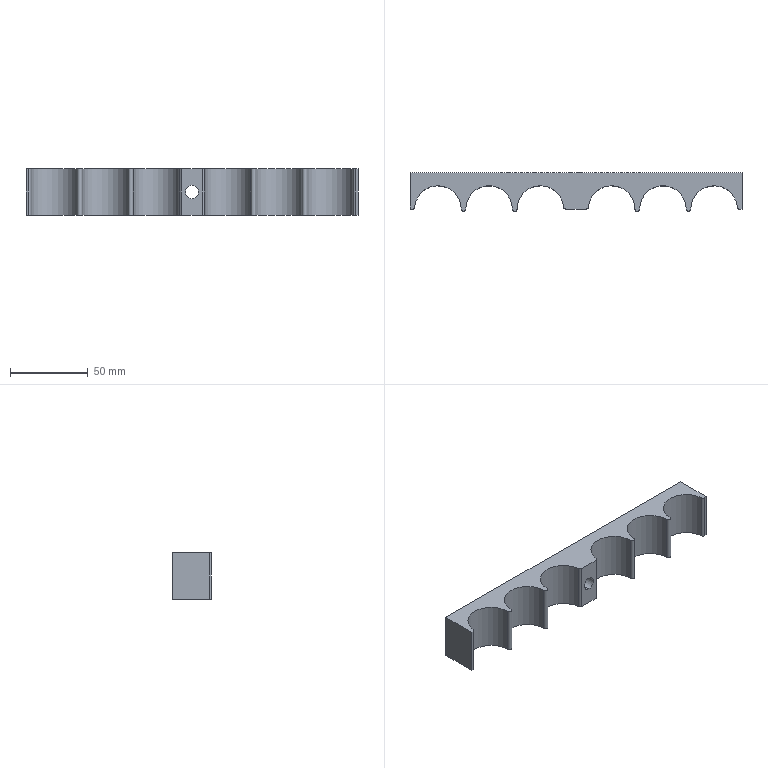Part | SolidWorks | features Extrusion 1, HoleWzd 1 | 1 solid | 24 faces | box 214 x 25 x 30 mm | volume 86293 mm3 | cylinder 16 | plane 8 | commonest cylinder face diameters 3 x8 30 x6 8.5 x2
STEP:
#1=CARTESIAN_POINT('',(0.,0.,10.75));
#2=VERTEX_POINT('',#1);
#3=CARTESIAN_POINT('',(0.,0.,19.25));
#4=VERTEX_POINT('',#3);
#5=CARTESIAN_POINT('',(0.,0.,15.));
#6=DIRECTION('',(0.,1.,0.));
#7=DIRECTION('',(0.,0.,1.));
#8=AXIS2_PLACEMENT_3D('',#5,#6,#7);
#9=CIRCLE('',#8,4.25);
#10=EDGE_CURVE('',#2,#4,#9,.T.);
#11=ORIENTED_EDGE('',*,*,#10,.F.);
#12=CARTESIAN_POINT('',(0.,23.5,10.75));
#13=VERTEX_POINT('',#12);
#14=CARTESIAN_POINT('',(0.,23.5,10.75));
#15=DIRECTION('',(0.,1.,0.));
#16=VECTOR('',#15,1000.);
#17=LINE('',#14,#16);
#18=EDGE_CURVE('',#2,#13,#17,.T.);
#19=ORIENTED_EDGE('',*,*,#18,.T.);
#20=CARTESIAN_POINT('',(0.,23.5,19.25));
#21=VERTEX_POINT('',#20);
#22=CARTESIAN_POINT('',(0.,23.5,15.));
#23=DIRECTION('',(0.,1.,0.));
#24=DIRECTION('',(0.,0.,1.));
#25=AXIS2_PLACEMENT_3D('',#22,#23,#24);
#26=CIRCLE('',#25,4.25);
#27=EDGE_CURVE('',#13,#21,#26,.T.);
#28=ORIENTED_EDGE('',*,*,#27,.T.);
#29=CARTESIAN_POINT('',(0.,23.5,19.25));
#30=DIRECTION('',(0.,1.,0.));
#31=VECTOR('',#30,1000.);
#32=LINE('',#29,#31);
#33=EDGE_CURVE('',#4,#21,#32,.T.);
#34=ORIENTED_EDGE('',*,*,#33,.F.);
#35=EDGE_LOOP('',(#11,#19,#28,#34));
#36=FACE_OUTER_BOUND('',#35,.T.);
#37=CARTESIAN_POINT('',(0.,23.5,15.));
#38=DIRECTION('',(0.,1.,0.));
#39=DIRECTION('',(0.,0.,1.));
#40=AXIS2_PLACEMENT_3D('',#37,#38,#39);
#41=CYLINDRICAL_SURFACE('',#40,4.25);
#42=ADVANCED_FACE('',(#36),#41,.F.);
#43=CARTESIAN_POINT('',(0.,23.5,15.));
#44=DIRECTION('',(0.,1.,0.));
#45=DIRECTION('',(0.,0.,1.));
#46=AXIS2_PLACEMENT_3D('',#43,#44,#45);
#47=CIRCLE('',#46,4.25);
#48=EDGE_CURVE('',#21,#13,#47,.T.);
#49=ORIENTED_EDGE('',*,*,#48,.F.);
#50=ORIENTED_EDGE('',*,*,#27,.F.);
#51=EDGE_LOOP('',(#49,#50));
#52=FACE_BOUND('',#51,.T.);
#53=CARTESIAN_POINT('',(107.,23.5,0.));
#54=VERTEX_POINT('',#53);
#55=CARTESIAN_POINT('',(-107.,23.5,0.));
#56=VERTEX_POINT('',#55);
#57=CARTESIAN_POINT('',(-107.,23.5,0.));
#58=DIRECTION('',(-1.,0.,0.));
#59=VECTOR('',#58,1000.);
#60=LINE('',#57,#59);
#61=EDGE_CURVE('',#54,#56,#60,.T.);
#62=ORIENTED_EDGE('',*,*,#61,.T.);
#63=CARTESIAN_POINT('',(-107.,23.5,30.));
#64=VERTEX_POINT('',#63);
#65=CARTESIAN_POINT('',(-107.,23.5,30.));
#66=DIRECTION('',(0.,0.,-1.));
#67=VECTOR('',#66,1000.);
#68=LINE('',#65,#67);
#69=EDGE_CURVE('',#64,#56,#68,.T.);
#70=ORIENTED_EDGE('',*,*,#69,.F.);
#71=CARTESIAN_POINT('',(107.,23.5,30.));
#72=VERTEX_POINT('',#71);
#73=CARTESIAN_POINT('',(-107.,23.5,30.));
#74=DIRECTION('',(-1.,0.,0.));
#75=VECTOR('',#74,1000.);
#76=LINE('',#73,#75);
#77=EDGE_CURVE('',#72,#64,#76,.T.);
#78=ORIENTED_EDGE('',*,*,#77,.F.);
#79=CARTESIAN_POINT('',(107.,23.5,30.));
#80=DIRECTION('',(0.,0.,-1.));
#81=VECTOR('',#80,1000.);
#82=LINE('',#79,#81);
#83=EDGE_CURVE('',#72,#54,#82,.T.);
#84=ORIENTED_EDGE('',*,*,#83,.T.);
#85=EDGE_LOOP('',(#62,#70,#78,#84));
#86=FACE_OUTER_BOUND('',#85,.T.);
#87=CARTESIAN_POINT('',(-107.,23.5,30.));
#88=DIRECTION('',(0.,-1.,0.));
#89=DIRECTION('',(1.,0.,0.));
#90=AXIS2_PLACEMENT_3D('',#87,#88,#89);
#91=PLANE('',#90);
#92=ADVANCED_FACE('',(#52,#86),#91,.F.);
#93=CARTESIAN_POINT('',(-107.,0.,0.));
#94=VERTEX_POINT('',#93);
#95=CARTESIAN_POINT('',(-107.,0.,0.));
#96=DIRECTION('',(0.,-1.,0.));
#97=VECTOR('',#96,1000.);
#98=LINE('',#95,#97);
#99=EDGE_CURVE('',#56,#94,#98,.T.);
#100=ORIENTED_EDGE('',*,*,#99,.T.);
#101=CARTESIAN_POINT('',(-107.,0.,30.));
#102=VERTEX_POINT('',#101);
#103=CARTESIAN_POINT('',(-107.,0.,30.));
#104=DIRECTION('',(0.,0.,-1.));
#105=VECTOR('',#104,1000.);
#106=LINE('',#103,#105);
#107=EDGE_CURVE('',#102,#94,#106,.T.);
#108=ORIENTED_EDGE('',*,*,#107,.F.);
#109=CARTESIAN_POINT('',(-107.,0.,30.));
#110=DIRECTION('',(0.,-1.,0.));
#111=VECTOR('',#110,1000.);
#112=LINE('',#109,#111);
#113=EDGE_CURVE('',#64,#102,#112,.T.);
#114=ORIENTED_EDGE('',*,*,#113,.F.);
#115=ORIENTED_EDGE('',*,*,#69,.T.);
#116=EDGE_LOOP('',(#100,#108,#114,#115));
#117=FACE_OUTER_BOUND('',#116,.T.);
#118=CARTESIAN_POINT('',(-107.,0.,30.));
#119=DIRECTION('',(1.,0.,0.));
#120=DIRECTION('',(0.,0.,-1.));
#121=AXIS2_PLACEMENT_3D('',#118,#119,#120);
#122=PLANE('',#121);
#123=ADVANCED_FACE('',(#117),#122,.F.);
#124=CARTESIAN_POINT('',(-105.432,0.,0.));
#125=VERTEX_POINT('',#124);
#126=CARTESIAN_POINT('',(-107.,0.,0.));
#127=DIRECTION('',(1.,0.,0.));
#128=VECTOR('',#127,1000.);
#129=LINE('',#126,#128);
#130=EDGE_CURVE('',#94,#125,#129,.T.);
#131=ORIENTED_EDGE('',*,*,#130,.T.);
#132=CARTESIAN_POINT('',(-105.432,0.,30.));
#133=VERTEX_POINT('',#132);
#134=CARTESIAN_POINT('',(-105.432,0.,30.));
#135=DIRECTION('',(0.,0.,-1.));
#136=VECTOR('',#135,1000.);
#137=LINE('',#134,#136);
#138=EDGE_CURVE('',#133,#125,#137,.T.);
#139=ORIENTED_EDGE('',*,*,#138,.F.);
#140=CARTESIAN_POINT('',(-107.,0.,30.));
#141=DIRECTION('',(1.,0.,0.));
#142=VECTOR('',#141,1000.);
#143=LINE('',#140,#142);
#144=EDGE_CURVE('',#102,#133,#143,.T.);
#145=ORIENTED_EDGE('',*,*,#144,.F.);
#146=ORIENTED_EDGE('',*,*,#107,.T.);
#147=EDGE_LOOP('',(#131,#139,#145,#146));
#148=FACE_OUTER_BOUND('',#147,.T.);
#149=CARTESIAN_POINT('',(-107.,0.,30.));
#150=DIRECTION('',(0.,1.,0.));
#151=DIRECTION('',(0.,0.,1.));
#152=AXIS2_PLACEMENT_3D('',#149,#150,#151);
#153=PLANE('',#152);
#154=ADVANCED_FACE('',(#148),#153,.F.);
#155=CARTESIAN_POINT('',(-103.938,1.364,0.));
#156=VERTEX_POINT('',#155);
#157=CARTESIAN_POINT('',(-105.432,1.5,0.));
#158=DIRECTION('',(0.,0.,1.));
#159=DIRECTION('',(1.,0.,0.));
#160=AXIS2_PLACEMENT_3D('',#157,#158,#159);
#161=CIRCLE('',#160,1.5);
#162=EDGE_CURVE('',#125,#156,#161,.T.);
#163=ORIENTED_EDGE('',*,*,#162,.T.);
#164=CARTESIAN_POINT('',(-103.938,1.364,30.));
#165=VERTEX_POINT('',#164);
#166=CARTESIAN_POINT('',(-103.938,1.364,30.));
#167=DIRECTION('',(0.,0.,-1.));
#168=VECTOR('',#167,1000.);
#169=LINE('',#166,#168);
#170=EDGE_CURVE('',#165,#156,#169,.T.);
#171=ORIENTED_EDGE('',*,*,#170,.F.);
#172=CARTESIAN_POINT('',(-105.432,1.5,30.));
#173=DIRECTION('',(0.,0.,1.));
#174=DIRECTION('',(1.,0.,0.));
#175=AXIS2_PLACEMENT_3D('',#172,#173,#174);
#176=CIRCLE('',#175,1.5);
#177=EDGE_CURVE('',#133,#165,#176,.T.);
#178=ORIENTED_EDGE('',*,*,#177,.F.);
#179=ORIENTED_EDGE('',*,*,#138,.T.);
#180=EDGE_LOOP('',(#163,#171,#178,#179));
#181=FACE_OUTER_BOUND('',#180,.T.);
#182=CARTESIAN_POINT('',(-105.432,1.5,30.));
#183=DIRECTION('',(0.,0.,-1.));
#184=DIRECTION('',(-1.,0.,0.));
#185=AXIS2_PLACEMENT_3D('',#182,#183,#184);
#186=CYLINDRICAL_SURFACE('',#185,1.5);
#187=ADVANCED_FACE('',(#181),#186,.T.);
#188=CARTESIAN_POINT('',(-74.,0.,0.));
#189=VERTEX_POINT('',#188);
#190=CARTESIAN_POINT('',(-89.,0.,0.));
#191=DIRECTION('',(0.,0.,-1.));
#192=DIRECTION('',(1.,0.,0.));
#193=AXIS2_PLACEMENT_3D('',#190,#191,#192);
#194=CIRCLE('',#193,15.);
#195=EDGE_CURVE('',#156,#189,#194,.T.);
#196=ORIENTED_EDGE('',*,*,#195,.T.);
#197=CARTESIAN_POINT('',(-74.,0.,30.));
#198=VERTEX_POINT('',#197);
#199=CARTESIAN_POINT('',(-74.,0.,30.));
#200=DIRECTION('',(0.,0.,-1.));
#201=VECTOR('',#200,1000.);
#202=LINE('',#199,#201);
#203=EDGE_CURVE('',#198,#189,#202,.T.);
#204=ORIENTED_EDGE('',*,*,#203,.F.);
#205=CARTESIAN_POINT('',(-89.,0.,30.));
#206=DIRECTION('',(0.,0.,-1.));
#207=DIRECTION('',(1.,0.,0.));
#208=AXIS2_PLACEMENT_3D('',#205,#206,#207);
#209=CIRCLE('',#208,15.);
#210=EDGE_CURVE('',#165,#198,#209,.T.);
#211=ORIENTED_EDGE('',*,*,#210,.F.);
#212=ORIENTED_EDGE('',*,*,#170,.T.);
#213=EDGE_LOOP('',(#196,#204,#211,#212));
#214=FACE_OUTER_BOUND('',#213,.T.);
#215=CARTESIAN_POINT('',(-89.,0.,30.));
#216=DIRECTION('',(0.,0.,-1.));
#217=DIRECTION('',(-1.,0.,0.));
#218=AXIS2_PLACEMENT_3D('',#215,#216,#217);
#219=CYLINDRICAL_SURFACE('',#218,15.);
#220=ADVANCED_FACE('',(#214),#219,.F.);
#221=CARTESIAN_POINT('',(-71.,0.,0.));
#222=VERTEX_POINT('',#221);
#223=CARTESIAN_POINT('',(-72.5,0.,0.));
#224=DIRECTION('',(0.,0.,1.));
#225=DIRECTION('',(1.,0.,0.));
#226=AXIS2_PLACEMENT_3D('',#223,#224,#225);
#227=CIRCLE('',#226,1.5);
#228=EDGE_CURVE('',#189,#222,#227,.T.);
#229=ORIENTED_EDGE('',*,*,#228,.T.);
#230=CARTESIAN_POINT('',(-71.,0.,30.));
#231=VERTEX_POINT('',#230);
#232=CARTESIAN_POINT('',(-71.,0.,30.));
#233=DIRECTION('',(0.,0.,-1.));
#234=VECTOR('',#233,1000.);
#235=LINE('',#232,#234);
#236=EDGE_CURVE('',#231,#222,#235,.T.);
#237=ORIENTED_EDGE('',*,*,#236,.F.);
#238=CARTESIAN_POINT('',(-72.5,0.,30.));
#239=DIRECTION('',(0.,0.,1.));
#240=DIRECTION('',(1.,0.,0.));
#241=AXIS2_PLACEMENT_3D('',#238,#239,#240);
#242=CIRCLE('',#241,1.5);
#243=EDGE_CURVE('',#198,#231,#242,.T.);
#244=ORIENTED_EDGE('',*,*,#243,.F.);
#245=ORIENTED_EDGE('',*,*,#203,.T.);
#246=EDGE_LOOP('',(#229,#237,#244,#245));
#247=FACE_OUTER_BOUND('',#246,.T.);
#248=CARTESIAN_POINT('',(-72.5,0.,30.));
#249=DIRECTION('',(0.,0.,-1.));
#250=DIRECTION('',(-1.,0.,0.));
#251=AXIS2_PLACEMENT_3D('',#248,#249,#250);
#252=CYLINDRICAL_SURFACE('',#251,1.5);
#253=ADVANCED_FACE('',(#247),#252,.T.);
#254=CARTESIAN_POINT('',(-41.,0.,0.));
#255=VERTEX_POINT('',#254);
#256=CARTESIAN_POINT('',(-56.,0.,0.));
#257=DIRECTION('',(0.,0.,-1.));
#258=DIRECTION('',(1.,0.,0.));
#259=AXIS2_PLACEMENT_3D('',#256,#257,#258);
#260=CIRCLE('',#259,15.);
#261=EDGE_CURVE('',#222,#255,#260,.T.);
#262=ORIENTED_EDGE('',*,*,#261,.T.);
#263=CARTESIAN_POINT('',(-41.,0.,30.));
#264=VERTEX_POINT('',#263);
#265=CARTESIAN_POINT('',(-41.,0.,30.));
#266=DIRECTION('',(0.,0.,-1.));
#267=VECTOR('',#266,1000.);
#268=LINE('',#265,#267);
#269=EDGE_CURVE('',#264,#255,#268,.T.);
#270=ORIENTED_EDGE('',*,*,#269,.F.);
#271=CARTESIAN_POINT('',(-56.,0.,30.));
#272=DIRECTION('',(0.,0.,-1.));
#273=DIRECTION('',(1.,0.,0.));
#274=AXIS2_PLACEMENT_3D('',#271,#272,#273);
#275=CIRCLE('',#274,15.);
#276=EDGE_CURVE('',#231,#264,#275,.T.);
#277=ORIENTED_EDGE('',*,*,#276,.F.);
#278=ORIENTED_EDGE('',*,*,#236,.T.);
#279=EDGE_LOOP('',(#262,#270,#277,#278));
#280=FACE_OUTER_BOUND('',#279,.T.);
#281=CARTESIAN_POINT('',(-56.,0.,30.));
#282=DIRECTION('',(0.,0.,-1.));
#283=DIRECTION('',(-1.,0.,0.));
#284=AXIS2_PLACEMENT_3D('',#281,#282,#283);
#285=CYLINDRICAL_SURFACE('',#284,15.);
#286=ADVANCED_FACE('',(#280),#285,.F.);
#287=CARTESIAN_POINT('',(-38.,0.,0.));
#288=VERTEX_POINT('',#287);
#289=CARTESIAN_POINT('',(-39.5,0.,0.));
#290=DIRECTION('',(0.,0.,1.));
#291=DIRECTION('',(1.,0.,0.));
#292=AXIS2_PLACEMENT_3D('',#289,#290,#291);
#293=CIRCLE('',#292,1.5);
#294=EDGE_CURVE('',#255,#288,#293,.T.);
#295=ORIENTED_EDGE('',*,*,#294,.T.);
#296=CARTESIAN_POINT('',(-38.,0.,30.));
#297=VERTEX_POINT('',#296);
#298=CARTESIAN_POINT('',(-38.,0.,30.));
#299=DIRECTION('',(0.,0.,-1.));
#300=VECTOR('',#299,1000.);
#301=LINE('',#298,#300);
#302=EDGE_CURVE('',#297,#288,#301,.T.);
#303=ORIENTED_EDGE('',*,*,#302,.F.);
#304=CARTESIAN_POINT('',(-39.5,0.,30.));
#305=DIRECTION('',(0.,0.,1.));
#306=DIRECTION('',(1.,0.,0.));
#307=AXIS2_PLACEMENT_3D('',#304,#305,#306);
#308=CIRCLE('',#307,1.5);
#309=EDGE_CURVE('',#264,#297,#308,.T.);
#310=ORIENTED_EDGE('',*,*,#309,.F.);
#311=ORIENTED_EDGE('',*,*,#269,.T.);
#312=EDGE_LOOP('',(#295,#303,#310,#311));
#313=FACE_OUTER_BOUND('',#312,.T.);
#314=CARTESIAN_POINT('',(-39.5,0.,30.));
#315=DIRECTION('',(0.,0.,-1.));
#316=DIRECTION('',(-1.,0.,0.));
#317=AXIS2_PLACEMENT_3D('',#314,#315,#316);
#318=CYLINDRICAL_SURFACE('',#317,1.5);
#319=ADVANCED_FACE('',(#313),#318,.T.);
#320=CARTESIAN_POINT('',(-8.062,1.364,0.));
#321=VERTEX_POINT('',#320);
#322=CARTESIAN_POINT('',(-23.,0.,0.));
#323=DIRECTION('',(0.,0.,-1.));
#324=DIRECTION('',(1.,0.,0.));
#325=AXIS2_PLACEMENT_3D('',#322,#323,#324);
#326=CIRCLE('',#325,15.);
#327=EDGE_CURVE('',#288,#321,#326,.T.);
#328=ORIENTED_EDGE('',*,*,#327,.T.);
#329=CARTESIAN_POINT('',(-8.062,1.364,30.));
#330=VERTEX_POINT('',#329);
#331=CARTESIAN_POINT('',(-8.062,1.364,30.));
#332=DIRECTION('',(0.,0.,-1.));
#333=VECTOR('',#332,1000.);
#334=LINE('',#331,#333);
#335=EDGE_CURVE('',#330,#321,#334,.T.);
#336=ORIENTED_EDGE('',*,*,#335,.F.);
#337=CARTESIAN_POINT('',(-23.,0.,30.));
#338=DIRECTION('',(0.,0.,-1.));
#339=DIRECTION('',(1.,0.,0.));
#340=AXIS2_PLACEMENT_3D('',#337,#338,#339);
#341=CIRCLE('',#340,15.);
#342=EDGE_CURVE('',#297,#330,#341,.T.);
#343=ORIENTED_EDGE('',*,*,#342,.F.);
#344=ORIENTED_EDGE('',*,*,#302,.T.);
#345=EDGE_LOOP('',(#328,#336,#343,#344));
#346=FACE_OUTER_BOUND('',#345,.T.);
#347=CARTESIAN_POINT('',(-23.,0.,30.));
#348=DIRECTION('',(0.,0.,-1.));
#349=DIRECTION('',(-1.,0.,0.));
#350=AXIS2_PLACEMENT_3D('',#347,#348,#349);
#351=CYLINDRICAL_SURFACE('',#350,15.);
#352=ADVANCED_FACE('',(#346),#351,.F.);
#353=CARTESIAN_POINT('',(-6.568,0.,0.));
#354=VERTEX_POINT('',#353);
#355=CARTESIAN_POINT('',(-6.568,1.5,0.));
#356=DIRECTION('',(0.,0.,1.));
#357=DIRECTION('',(1.,0.,0.));
#358=AXIS2_PLACEMENT_3D('',#355,#356,#357);
#359=CIRCLE('',#358,1.5);
#360=EDGE_CURVE('',#321,#354,#359,.T.);
#361=ORIENTED_EDGE('',*,*,#360,.T.);
#362=CARTESIAN_POINT('',(-6.568,0.,30.));
#363=VERTEX_POINT('',#362);
#364=CARTESIAN_POINT('',(-6.568,0.,30.));
#365=DIRECTION('',(0.,0.,-1.));
#366=VECTOR('',#365,1000.);
#367=LINE('',#364,#366);
#368=EDGE_CURVE('',#363,#354,#367,.T.);
#369=ORIENTED_EDGE('',*,*,#368,.F.);
#370=CARTESIAN_POINT('',(-6.568,1.5,30.));
#371=DIRECTION('',(0.,0.,1.));
#372=DIRECTION('',(1.,0.,0.));
#373=AXIS2_PLACEMENT_3D('',#370,#371,#372);
#374=CIRCLE('',#373,1.5);
#375=EDGE_CURVE('',#330,#363,#374,.T.);
#376=ORIENTED_EDGE('',*,*,#375,.F.);
#377=ORIENTED_EDGE('',*,*,#335,.T.);
#378=EDGE_LOOP('',(#361,#369,#376,#377));
#379=FACE_OUTER_BOUND('',#378,.T.);
#380=CARTESIAN_POINT('',(-6.568,1.5,30.));
#381=DIRECTION('',(0.,0.,-1.));
#382=DIRECTION('',(-1.,0.,0.));
#383=AXIS2_PLACEMENT_3D('',#380,#381,#382);
#384=CYLINDRICAL_SURFACE('',#383,1.5);
#385=ADVANCED_FACE('',(#379),#384,.T.);
#386=CARTESIAN_POINT('',(0.,0.,15.));
#387=DIRECTION('',(0.,1.,0.));
#388=DIRECTION('',(0.,0.,1.));
#389=AXIS2_PLACEMENT_3D('',#386,#387,#388);
#390=CIRCLE('',#389,4.25);
#391=EDGE_CURVE('',#4,#2,#390,.T.);
#392=ORIENTED_EDGE('',*,*,#391,.T.);
#393=ORIENTED_EDGE('',*,*,#10,.T.);
#394=EDGE_LOOP('',(#392,#393));
#395=FACE_BOUND('',#394,.T.);
#396=CARTESIAN_POINT('',(6.568,0.,0.));
#397=VERTEX_POINT('',#396);
#398=CARTESIAN_POINT('',(6.568,0.,0.));
#399=DIRECTION('',(1.,0.,0.));
#400=VECTOR('',#399,1000.);
#401=LINE('',#398,#400);
#402=EDGE_CURVE('',#354,#397,#401,.T.);
#403=ORIENTED_EDGE('',*,*,#402,.T.);
#404=CARTESIAN_POINT('',(6.568,0.,30.));
#405=VERTEX_POINT('',#404);
#406=CARTESIAN_POINT('',(6.568,0.,30.));
#407=DIRECTION('',(0.,0.,-1.));
#408=VECTOR('',#407,1000.);
#409=LINE('',#406,#408);
#410=EDGE_CURVE('',#405,#397,#409,.T.);
#411=ORIENTED_EDGE('',*,*,#410,.F.);
#412=CARTESIAN_POINT('',(6.568,0.,30.));
#413=DIRECTION('',(1.,0.,0.));
#414=VECTOR('',#413,1000.);
#415=LINE('',#412,#414);
#416=EDGE_CURVE('',#363,#405,#415,.T.);
#417=ORIENTED_EDGE('',*,*,#416,.F.);
#418=ORIENTED_EDGE('',*,*,#368,.T.);
#419=EDGE_LOOP('',(#403,#411,#417,#418));
#420=FACE_OUTER_BOUND('',#419,.T.);
#421=CARTESIAN_POINT('',(6.568,0.,30.));
#422=DIRECTION('',(0.,1.,0.));
#423=DIRECTION('',(0.,0.,1.));
#424=AXIS2_PLACEMENT_3D('',#421,#422,#423);
#425=PLANE('',#424);
#426=ADVANCED_FACE('',(#395,#420),#425,.F.);
#427=CARTESIAN_POINT('',(8.062,1.364,0.));
#428=VERTEX_POINT('',#427);
#429=CARTESIAN_POINT('',(6.568,1.5,0.));
#430=DIRECTION('',(0.,0.,1.));
#431=DIRECTION('',(-1.,0.,0.));
#432=AXIS2_PLACEMENT_3D('',#429,#430,#431);
#433=CIRCLE('',#432,1.5);
#434=EDGE_CURVE('',#397,#428,#433,.T.);
#435=ORIENTED_EDGE('',*,*,#434,.T.);
#436=CARTESIAN_POINT('',(8.062,1.364,30.));
#437=VERTEX_POINT('',#436);
#438=CARTESIAN_POINT('',(8.062,1.364,30.));
#439=DIRECTION('',(0.,0.,-1.));
#440=VECTOR('',#439,1000.);
#441=LINE('',#438,#440);
#442=EDGE_CURVE('',#437,#428,#441,.T.);
#443=ORIENTED_EDGE('',*,*,#442,.F.);
#444=CARTESIAN_POINT('',(6.568,1.5,30.));
#445=DIRECTION('',(0.,0.,1.));
#446=DIRECTION('',(-1.,0.,0.));
#447=AXIS2_PLACEMENT_3D('',#444,#445,#446);
#448=CIRCLE('',#447,1.5);
#449=EDGE_CURVE('',#405,#437,#448,.T.);
#450=ORIENTED_EDGE('',*,*,#449,.F.);
#451=ORIENTED_EDGE('',*,*,#410,.T.);
#452=EDGE_LOOP('',(#435,#443,#450,#451));
#453=FACE_OUTER_BOUND('',#452,.T.);
#454=CARTESIAN_POINT('',(6.568,1.5,30.));
#455=DIRECTION('',(0.,0.,-1.));
#456=DIRECTION('',(-1.,0.,0.));
#457=AXIS2_PLACEMENT_3D('',#454,#455,#456);
#458=CYLINDRICAL_SURFACE('',#457,1.5);
#459=ADVANCED_FACE('',(#453),#458,.T.);
#460=CARTESIAN_POINT('',(38.,0.,0.));
#461=VERTEX_POINT('',#460);
#462=CARTESIAN_POINT('',(23.,0.,0.));
#463=DIRECTION('',(0.,0.,-1.));
#464=DIRECTION('',(-1.,0.,0.));
#465=AXIS2_PLACEMENT_3D('',#462,#463,#464);
#466=CIRCLE('',#465,15.);
#467=EDGE_CURVE('',#428,#461,#466,.T.);
#468=ORIENTED_EDGE('',*,*,#467,.T.);
#469=CARTESIAN_POINT('',(38.,0.,30.));
#470=VERTEX_POINT('',#469);
#471=CARTESIAN_POINT('',(38.,0.,30.));
#472=DIRECTION('',(0.,0.,-1.));
#473=VECTOR('',#472,1000.);
#474=LINE('',#471,#473);
#475=EDGE_CURVE('',#470,#461,#474,.T.);
#476=ORIENTED_EDGE('',*,*,#475,.F.);
#477=CARTESIAN_POINT('',(23.,0.,30.));
#478=DIRECTION('',(0.,0.,-1.));
#479=DIRECTION('',(-1.,0.,0.));
#480=AXIS2_PLACEMENT_3D('',#477,#478,#479);
#481=CIRCLE('',#480,15.);
#482=EDGE_CURVE('',#437,#470,#481,.T.);
#483=ORIENTED_EDGE('',*,*,#482,.F.);
#484=ORIENTED_EDGE('',*,*,#442,.T.);
#485=EDGE_LOOP('',(#468,#476,#483,#484));
#486=FACE_OUTER_BOUND('',#485,.T.);
#487=CARTESIAN_POINT('',(23.,0.,30.));
#488=DIRECTION('',(0.,0.,-1.));
#489=DIRECTION('',(-1.,0.,0.));
#490=AXIS2_PLACEMENT_3D('',#487,#488,#489);
#491=CYLINDRICAL_SURFACE('',#490,15.);
#492=ADVANCED_FACE('',(#486),#491,.F.);
#493=CARTESIAN_POINT('',(41.,0.,0.));
#494=VERTEX_POINT('',#493);
#495=CARTESIAN_POINT('',(39.5,0.,0.));
#496=DIRECTION('',(0.,0.,1.));
#497=DIRECTION('',(-1.,0.,0.));
#498=AXIS2_PLACEMENT_3D('',#495,#496,#497);
#499=CIRCLE('',#498,1.5);
#500=EDGE_CURVE('',#461,#494,#499,.T.);
#501=ORIENTED_EDGE('',*,*,#500,.T.);
#502=CARTESIAN_POINT('',(41.,0.,30.));
#503=VERTEX_POINT('',#502);
#504=CARTESIAN_POINT('',(41.,0.,30.));
#505=DIRECTION('',(0.,0.,-1.));
#506=VECTOR('',#505,1000.);
#507=LINE('',#504,#506);
#508=EDGE_CURVE('',#503,#494,#507,.T.);
#509=ORIENTED_EDGE('',*,*,#508,.F.);
#510=CARTESIAN_POINT('',(39.5,0.,30.));
#511=DIRECTION('',(0.,0.,1.));
#512=DIRECTION('',(-1.,0.,0.));
#513=AXIS2_PLACEMENT_3D('',#510,#511,#512);
#514=CIRCLE('',#513,1.5);
#515=EDGE_CURVE('',#470,#503,#514,.T.);
#516=ORIENTED_EDGE('',*,*,#515,.F.);
#517=ORIENTED_EDGE('',*,*,#475,.T.);
#518=EDGE_LOOP('',(#501,#509,#516,#517));
#519=FACE_OUTER_BOUND('',#518,.T.);
#520=CARTESIAN_POINT('',(39.5,0.,30.));
#521=DIRECTION('',(0.,0.,-1.));
#522=DIRECTION('',(-1.,0.,0.));
#523=AXIS2_PLACEMENT_3D('',#520,#521,#522);
#524=CYLINDRICAL_SURFACE('',#523,1.5);
#525=ADVANCED_FACE('',(#519),#524,.T.);
#526=CARTESIAN_POINT('',(71.,0.,0.));
#527=VERTEX_POINT('',#526);
#528=CARTESIAN_POINT('',(56.,0.,0.));
#529=DIRECTION('',(0.,0.,-1.));
#530=DIRECTION('',(-1.,0.,0.));
#531=AXIS2_PLACEMENT_3D('',#528,#529,#530);
#532=CIRCLE('',#531,15.);
#533=EDGE_CURVE('',#494,#527,#532,.T.);
#534=ORIENTED_EDGE('',*,*,#533,.T.);
#535=CARTESIAN_POINT('',(71.,0.,30.));
#536=VERTEX_POINT('',#535);
#537=CARTESIAN_POINT('',(71.,0.,30.));
#538=DIRECTION('',(0.,0.,-1.));
#539=VECTOR('',#538,1000.);
#540=LINE('',#537,#539);
#541=EDGE_CURVE('',#536,#527,#540,.T.);
#542=ORIENTED_EDGE('',*,*,#541,.F.);
#543=CARTESIAN_POINT('',(56.,0.,30.));
#544=DIRECTION('',(0.,0.,-1.));
#545=DIRECTION('',(-1.,0.,0.));
#546=AXIS2_PLACEMENT_3D('',#543,#544,#545);
#547=CIRCLE('',#546,15.);
#548=EDGE_CURVE('',#503,#536,#547,.T.);
#549=ORIENTED_EDGE('',*,*,#548,.F.);
#550=ORIENTED_EDGE('',*,*,#508,.T.);
#551=EDGE_LOOP('',(#534,#542,#549,#550));
#552=FACE_OUTER_BOUND('',#551,.T.);
#553=CARTESIAN_POINT('',(56.,0.,30.));
#554=DIRECTION('',(0.,0.,-1.));
#555=DIRECTION('',(-1.,0.,0.));
#556=AXIS2_PLACEMENT_3D('',#553,#554,#555);
#557=CYLINDRICAL_SURFACE('',#556,15.);
#558=ADVANCED_FACE('',(#552),#557,.F.);
#559=CARTESIAN_POINT('',(74.,0.,0.));
#560=VERTEX_POINT('',#559);
#561=CARTESIAN_POINT('',(72.5,0.,0.));
#562=DIRECTION('',(0.,0.,1.));
#563=DIRECTION('',(-1.,0.,0.));
#564=AXIS2_PLACEMENT_3D('',#561,#562,#563);
#565=CIRCLE('',#564,1.5);
#566=EDGE_CURVE('',#527,#560,#565,.T.);
#567=ORIENTED_EDGE('',*,*,#566,.T.);
#568=CARTESIAN_POINT('',(74.,0.,30.));
#569=VERTEX_POINT('',#568);
#570=CARTESIAN_POINT('',(74.,0.,30.));
#571=DIRECTION('',(0.,0.,-1.));
#572=VECTOR('',#571,1000.);
#573=LINE('',#570,#572);
#574=EDGE_CURVE('',#569,#560,#573,.T.);
#575=ORIENTED_EDGE('',*,*,#574,.F.);
#576=CARTESIAN_POINT('',(72.5,0.,30.));
#577=DIRECTION('',(0.,0.,1.));
#578=DIRECTION('',(-1.,0.,0.));
#579=AXIS2_PLACEMENT_3D('',#576,#577,#578);
#580=CIRCLE('',#579,1.5);
#581=EDGE_CURVE('',#536,#569,#580,.T.);
#582=ORIENTED_EDGE('',*,*,#581,.F.);
#583=ORIENTED_EDGE('',*,*,#541,.T.);
#584=EDGE_LOOP('',(#567,#575,#582,#583));
#585=FACE_OUTER_BOUND('',#584,.T.);
#586=CARTESIAN_POINT('',(72.5,0.,30.));
#587=DIRECTION('',(0.,0.,-1.));
#588=DIRECTION('',(-1.,0.,0.));
#589=AXIS2_PLACEMENT_3D('',#586,#587,#588);
#590=CYLINDRICAL_SURFACE('',#589,1.5);
#591=ADVANCED_FACE('',(#585),#590,.T.);
#592=CARTESIAN_POINT('',(103.938,1.364,0.));
#593=VERTEX_POINT('',#592);
#594=CARTESIAN_POINT('',(89.,0.,0.));
#595=DIRECTION('',(0.,0.,-1.));
#596=DIRECTION('',(-1.,0.,0.));
#597=AXIS2_PLACEMENT_3D('',#594,#595,#596);
#598=CIRCLE('',#597,15.);
#599=EDGE_CURVE('',#560,#593,#598,.T.);
#600=ORIENTED_EDGE('',*,*,#599,.T.);
#601=CARTESIAN_POINT('',(103.938,1.364,30.));
#602=VERTEX_POINT('',#601);
#603=CARTESIAN_POINT('',(103.938,1.364,30.));
#604=DIRECTION('',(0.,0.,-1.));
#605=VECTOR('',#604,1000.);
#606=LINE('',#603,#605);
#607=EDGE_CURVE('',#602,#593,#606,.T.);
#608=ORIENTED_EDGE('',*,*,#607,.F.);
#609=CARTESIAN_POINT('',(89.,0.,30.));
#610=DIRECTION('',(0.,0.,-1.));
#611=DIRECTION('',(-1.,0.,0.));
#612=AXIS2_PLACEMENT_3D('',#609,#610,#611);
#613=CIRCLE('',#612,15.);
#614=EDGE_CURVE('',#569,#602,#613,.T.);
#615=ORIENTED_EDGE('',*,*,#614,.F.);
#616=ORIENTED_EDGE('',*,*,#574,.T.);
#617=EDGE_LOOP('',(#600,#608,#615,#616));
#618=FACE_OUTER_BOUND('',#617,.T.);
#619=CARTESIAN_POINT('',(89.,0.,30.));
#620=DIRECTION('',(0.,0.,-1.));
#621=DIRECTION('',(-1.,0.,0.));
#622=AXIS2_PLACEMENT_3D('',#619,#620,#621);
#623=CYLINDRICAL_SURFACE('',#622,15.);
#624=ADVANCED_FACE('',(#618),#623,.F.);
#625=CARTESIAN_POINT('',(105.432,0.,0.));
#626=VERTEX_POINT('',#625);
#627=CARTESIAN_POINT('',(105.432,1.5,0.));
#628=DIRECTION('',(0.,0.,1.));
#629=DIRECTION('',(-1.,0.,0.));
#630=AXIS2_PLACEMENT_3D('',#627,#628,#629);
#631=CIRCLE('',#630,1.5);
#632=EDGE_CURVE('',#593,#626,#631,.T.);
#633=ORIENTED_EDGE('',*,*,#632,.T.);
#634=CARTESIAN_POINT('',(105.432,0.,30.));
#635=VERTEX_POINT('',#634);
#636=CARTESIAN_POINT('',(105.432,0.,30.));
#637=DIRECTION('',(0.,0.,-1.));
#638=VECTOR('',#637,1000.);
#639=LINE('',#636,#638);
#640=EDGE_CURVE('',#635,#626,#639,.T.);
#641=ORIENTED_EDGE('',*,*,#640,.F.);
#642=CARTESIAN_POINT('',(105.432,1.5,30.));
#643=DIRECTION('',(0.,0.,1.));
#644=DIRECTION('',(-1.,0.,0.));
#645=AXIS2_PLACEMENT_3D('',#642,#643,#644);
#646=CIRCLE('',#645,1.5);
#647=EDGE_CURVE('',#602,#635,#646,.T.);
#648=ORIENTED_EDGE('',*,*,#647,.F.);
#649=ORIENTED_EDGE('',*,*,#607,.T.);
#650=EDGE_LOOP('',(#633,#641,#648,#649));
#651=FACE_OUTER_BOUND('',#650,.T.);
#652=CARTESIAN_POINT('',(105.432,1.5,30.));
#653=DIRECTION('',(0.,0.,-1.));
#654=DIRECTION('',(-1.,0.,0.));
#655=AXIS2_PLACEMENT_3D('',#652,#653,#654);
#656=CYLINDRICAL_SURFACE('',#655,1.5);
#657=ADVANCED_FACE('',(#651),#656,.T.);
#658=CARTESIAN_POINT('',(107.,0.,0.));
#659=VERTEX_POINT('',#658);
#660=CARTESIAN_POINT('',(107.,0.,0.));
#661=DIRECTION('',(1.,0.,0.));
#662=VECTOR('',#661,1000.);
#663=LINE('',#660,#662);
#664=EDGE_CURVE('',#626,#659,#663,.T.);
#665=ORIENTED_EDGE('',*,*,#664,.T.);
#666=CARTESIAN_POINT('',(107.,0.,30.));
#667=VERTEX_POINT('',#666);
#668=CARTESIAN_POINT('',(107.,0.,30.));
#669=DIRECTION('',(0.,0.,-1.));
#670=VECTOR('',#669,1000.);
#671=LINE('',#668,#670);
#672=EDGE_CURVE('',#667,#659,#671,.T.);
#673=ORIENTED_EDGE('',*,*,#672,.F.);
#674=CARTESIAN_POINT('',(107.,0.,30.));
#675=DIRECTION('',(1.,0.,0.));
#676=VECTOR('',#675,1000.);
#677=LINE('',#674,#676);
#678=EDGE_CURVE('',#635,#667,#677,.T.);
#679=ORIENTED_EDGE('',*,*,#678,.F.);
#680=ORIENTED_EDGE('',*,*,#640,.T.);
#681=EDGE_LOOP('',(#665,#673,#679,#680));
#682=FACE_OUTER_BOUND('',#681,.T.);
#683=CARTESIAN_POINT('',(107.,0.,30.));
#684=DIRECTION('',(0.,1.,0.));
#685=DIRECTION('',(0.,0.,1.));
#686=AXIS2_PLACEMENT_3D('',#683,#684,#685);
#687=PLANE('',#686);
#688=ADVANCED_FACE('',(#682),#687,.F.);
#689=CARTESIAN_POINT('',(107.,0.,0.));
#690=DIRECTION('',(0.,1.,0.));
#691=VECTOR('',#690,1000.);
#692=LINE('',#689,#691);
#693=EDGE_CURVE('',#659,#54,#692,.T.);
#694=ORIENTED_EDGE('',*,*,#693,.T.);
#695=ORIENTED_EDGE('',*,*,#83,.F.);
#696=CARTESIAN_POINT('',(107.,0.,30.));
#697=DIRECTION('',(0.,1.,0.));
#698=VECTOR('',#697,1000.);
#699=LINE('',#696,#698);
#700=EDGE_CURVE('',#667,#72,#699,.T.);
#701=ORIENTED_EDGE('',*,*,#700,.F.);
#702=ORIENTED_EDGE('',*,*,#672,.T.);
#703=EDGE_LOOP('',(#694,#695,#701,#702));
#704=FACE_OUTER_BOUND('',#703,.T.);
#705=CARTESIAN_POINT('',(107.,0.,30.));
#706=DIRECTION('',(-1.,0.,0.));
#707=DIRECTION('',(0.,0.,1.));
#708=AXIS2_PLACEMENT_3D('',#705,#706,#707);
#709=PLANE('',#708);
#710=ADVANCED_FACE('',(#704),#709,.F.);
#711=ORIENTED_EDGE('',*,*,#77,.T.);
#712=ORIENTED_EDGE('',*,*,#113,.T.);
#713=ORIENTED_EDGE('',*,*,#144,.T.);
#714=ORIENTED_EDGE('',*,*,#177,.T.);
#715=ORIENTED_EDGE('',*,*,#210,.T.);
#716=ORIENTED_EDGE('',*,*,#243,.T.);
#717=ORIENTED_EDGE('',*,*,#276,.T.);
#718=ORIENTED_EDGE('',*,*,#309,.T.);
#719=ORIENTED_EDGE('',*,*,#342,.T.);
#720=ORIENTED_EDGE('',*,*,#375,.T.);
#721=ORIENTED_EDGE('',*,*,#416,.T.);
#722=ORIENTED_EDGE('',*,*,#449,.T.);
#723=ORIENTED_EDGE('',*,*,#482,.T.);
#724=ORIENTED_EDGE('',*,*,#515,.T.);
#725=ORIENTED_EDGE('',*,*,#548,.T.);
#726=ORIENTED_EDGE('',*,*,#581,.T.);
#727=ORIENTED_EDGE('',*,*,#614,.T.);
#728=ORIENTED_EDGE('',*,*,#647,.T.);
#729=ORIENTED_EDGE('',*,*,#678,.T.);
#730=ORIENTED_EDGE('',*,*,#700,.T.);
#731=EDGE_LOOP('',(#711,#712,#713,#714,#715,#716,#717,#718,#719,#720,#721,#722,#723,#724,#725,#726,#727,#728,#729,#730));
#732=FACE_OUTER_BOUND('',#731,.T.);
#733=CARTESIAN_POINT('',(105.432,1.5,30.));
#734=DIRECTION('',(0.,0.,-1.));
#735=DIRECTION('',(-1.,0.,0.));
#736=AXIS2_PLACEMENT_3D('',#733,#734,#735);
#737=PLANE('',#736);
#738=ADVANCED_FACE('',(#732),#737,.F.);
#739=ORIENTED_EDGE('',*,*,#61,.F.);
#740=ORIENTED_EDGE('',*,*,#693,.F.);
#741=ORIENTED_EDGE('',*,*,#664,.F.);
#742=ORIENTED_EDGE('',*,*,#632,.F.);
#743=ORIENTED_EDGE('',*,*,#599,.F.);
#744=ORIENTED_EDGE('',*,*,#566,.F.);
#745=ORIENTED_EDGE('',*,*,#533,.F.);
#746=ORIENTED_EDGE('',*,*,#500,.F.);
#747=ORIENTED_EDGE('',*,*,#467,.F.);
#748=ORIENTED_EDGE('',*,*,#434,.F.);
#749=ORIENTED_EDGE('',*,*,#402,.F.);
#750=ORIENTED_EDGE('',*,*,#360,.F.);
#751=ORIENTED_EDGE('',*,*,#327,.F.);
#752=ORIENTED_EDGE('',*,*,#294,.F.);
#753=ORIENTED_EDGE('',*,*,#261,.F.);
#754=ORIENTED_EDGE('',*,*,#228,.F.);
#755=ORIENTED_EDGE('',*,*,#195,.F.);
#756=ORIENTED_EDGE('',*,*,#162,.F.);
#757=ORIENTED_EDGE('',*,*,#130,.F.);
#758=ORIENTED_EDGE('',*,*,#99,.F.);
#759=EDGE_LOOP('',(#739,#740,#741,#742,#743,#744,#745,#746,#747,#748,#749,#750,#751,#752,#753,#754,#755,#756,#757,#758));
#760=FACE_OUTER_BOUND('',#759,.T.);
#761=CARTESIAN_POINT('',(105.432,1.5,0.));
#762=DIRECTION('',(0.,0.,-1.));
#763=DIRECTION('',(-1.,0.,0.));
#764=AXIS2_PLACEMENT_3D('',#761,#762,#763);
#765=PLANE('',#764);
#766=ADVANCED_FACE('',(#760),#765,.T.);
#767=ORIENTED_EDGE('',*,*,#18,.F.);
#768=ORIENTED_EDGE('',*,*,#391,.F.);
#769=ORIENTED_EDGE('',*,*,#33,.T.);
#770=ORIENTED_EDGE('',*,*,#48,.T.);
#771=EDGE_LOOP('',(#767,#768,#769,#770));
#772=FACE_OUTER_BOUND('',#771,.T.);
#773=CARTESIAN_POINT('',(0.,23.5,15.));
#774=DIRECTION('',(0.,1.,0.));
#775=DIRECTION('',(0.,0.,1.));
#776=AXIS2_PLACEMENT_3D('',#773,#774,#775);
#777=CYLINDRICAL_SURFACE('',#776,4.25);
#778=ADVANCED_FACE('',(#772),#777,.F.);
#779=CLOSED_SHELL('',(#42,#92,#123,#154,#187,#220,#253,#286,#319,#352,#385,#426,#459,#492,#525,#558,#591,#624,#657,#688,#710,#738,#766,#778));
#780=MANIFOLD_SOLID_BREP('',#779);
#781=CARTESIAN_POINT('',(0.,0.,0.));
#782=DIRECTION('',(0.,0.,1.));
#783=DIRECTION('',(1.,0.,0.));
#784=AXIS2_PLACEMENT_3D('',#781,#782,#783);
#785=(LENGTH_UNIT()NAMED_UNIT(*)SI_UNIT(.MILLI.,.METRE.));
#786=UNCERTAINTY_MEASURE_WITH_UNIT(LENGTH_MEASURE(0.00001),#785,'','');
#787=(NAMED_UNIT(*)PLANE_ANGLE_UNIT()SI_UNIT($,.RADIAN.));
#788=(NAMED_UNIT(*)SI_UNIT($,.STERADIAN.)SOLID_ANGLE_UNIT());
#789=(GEOMETRIC_REPRESENTATION_CONTEXT(3)GLOBAL_UNCERTAINTY_ASSIGNED_CONTEXT((#786))GLOBAL_UNIT_ASSIGNED_CONTEXT((#785,#787,#788))REPRESENTATION_CONTEXT('',''));
#790=ADVANCED_BREP_SHAPE_REPRESENTATION('',(#780,#784),#789);